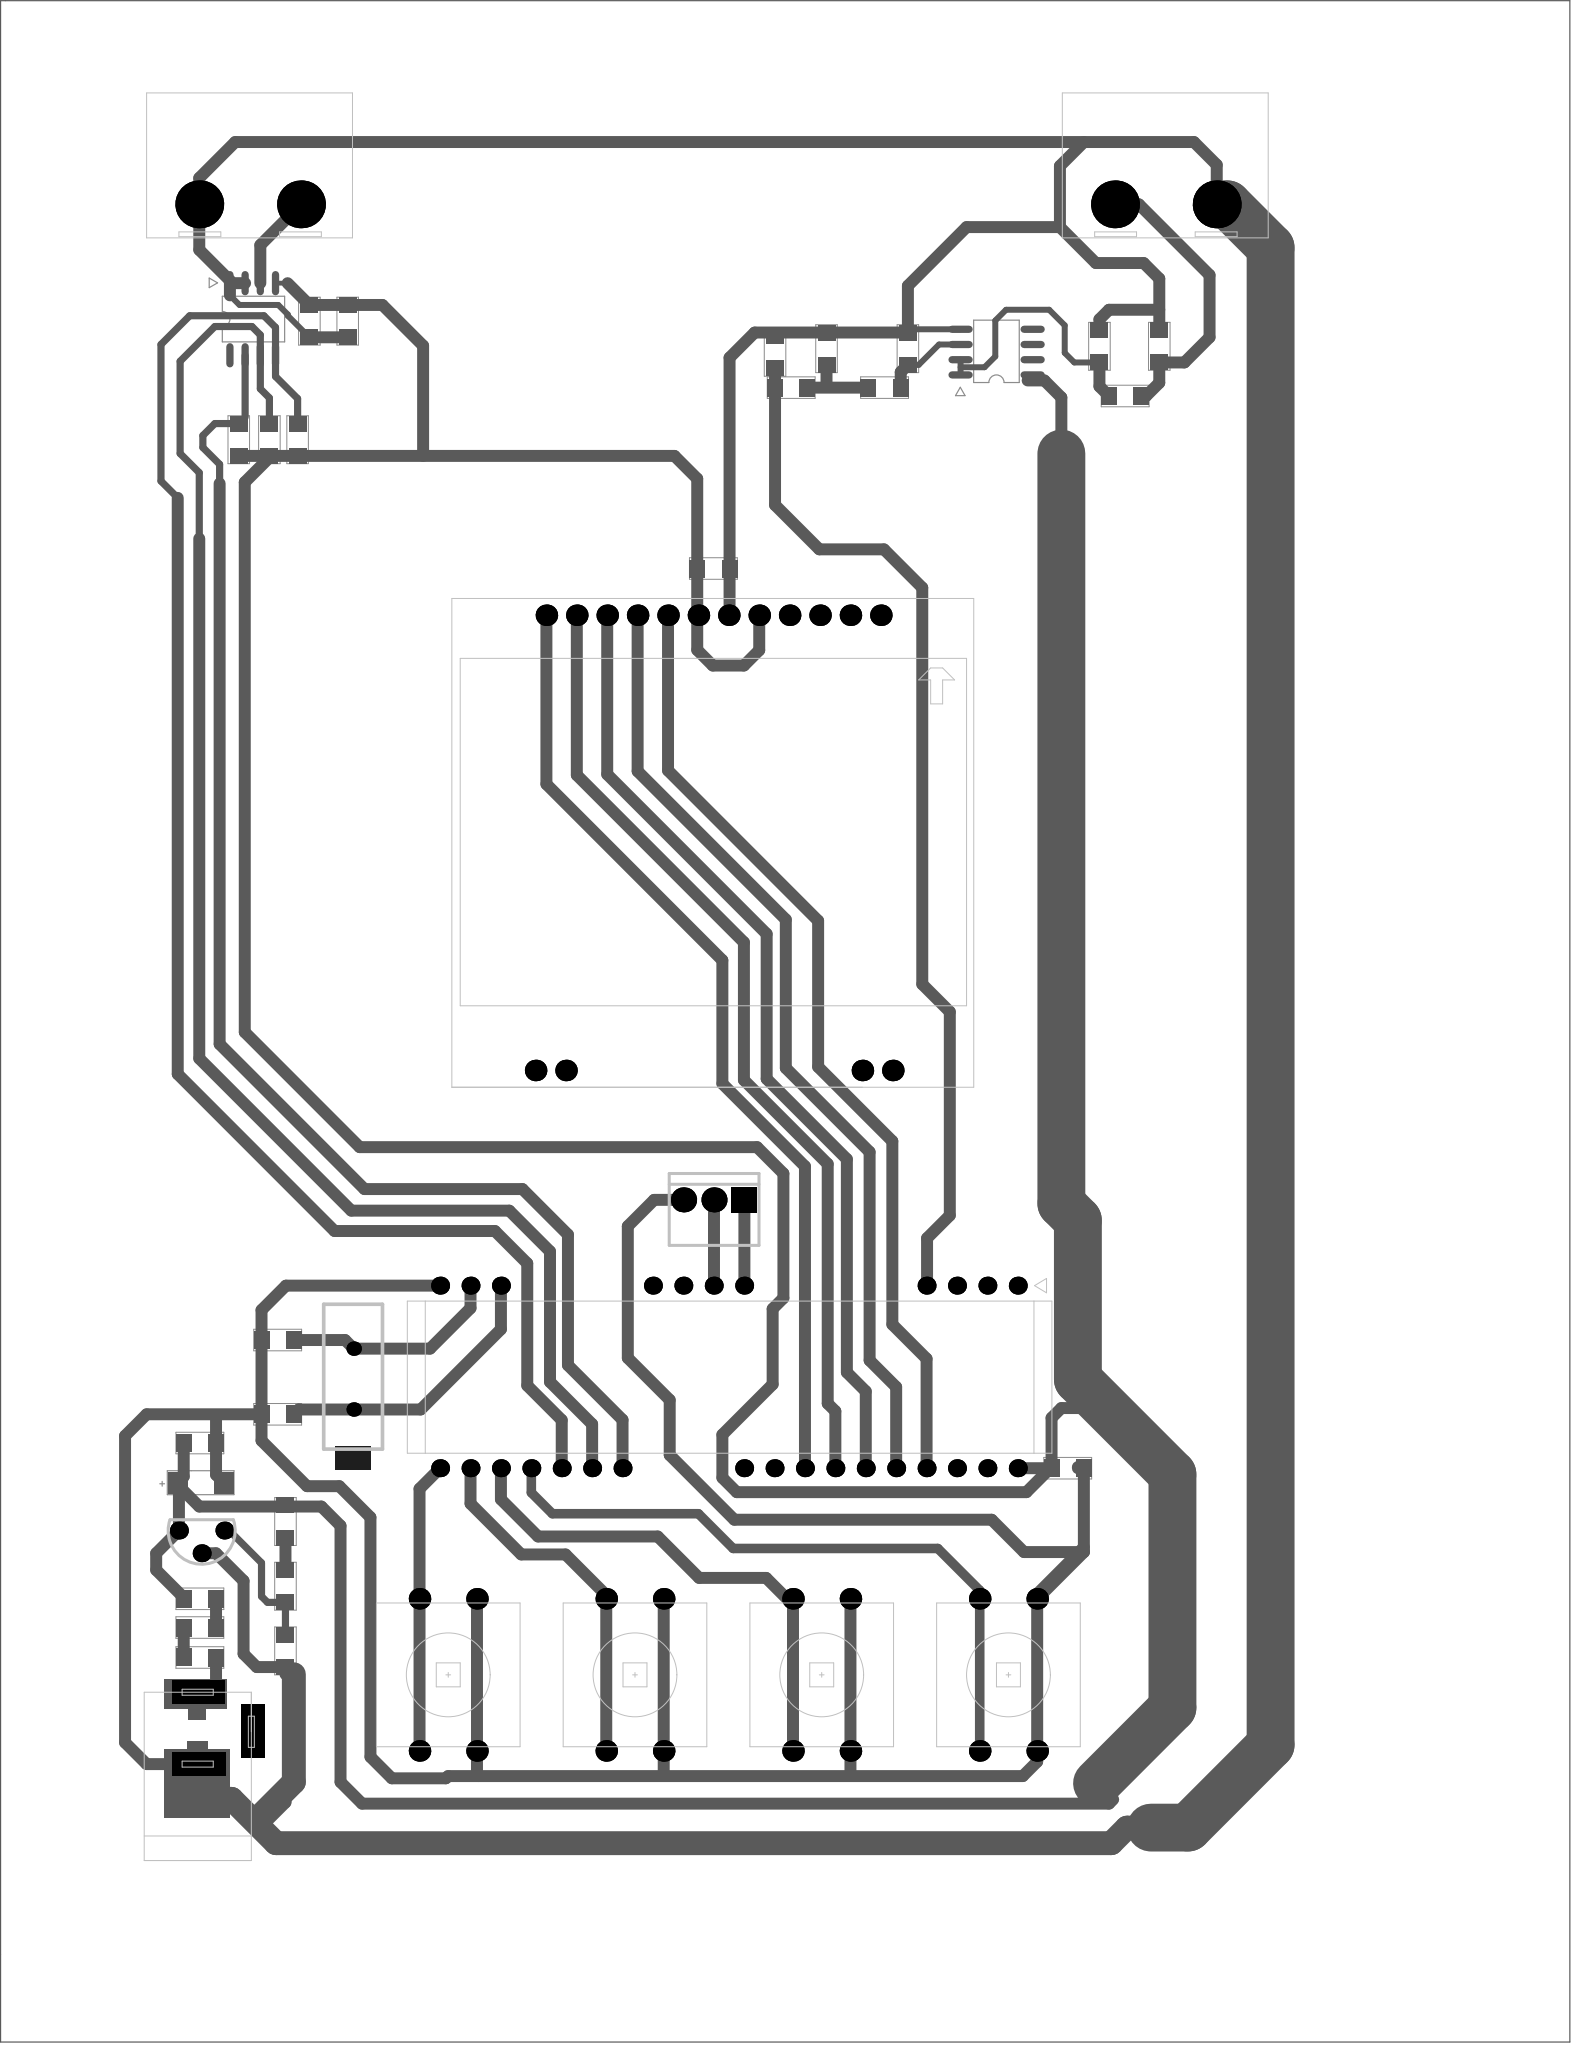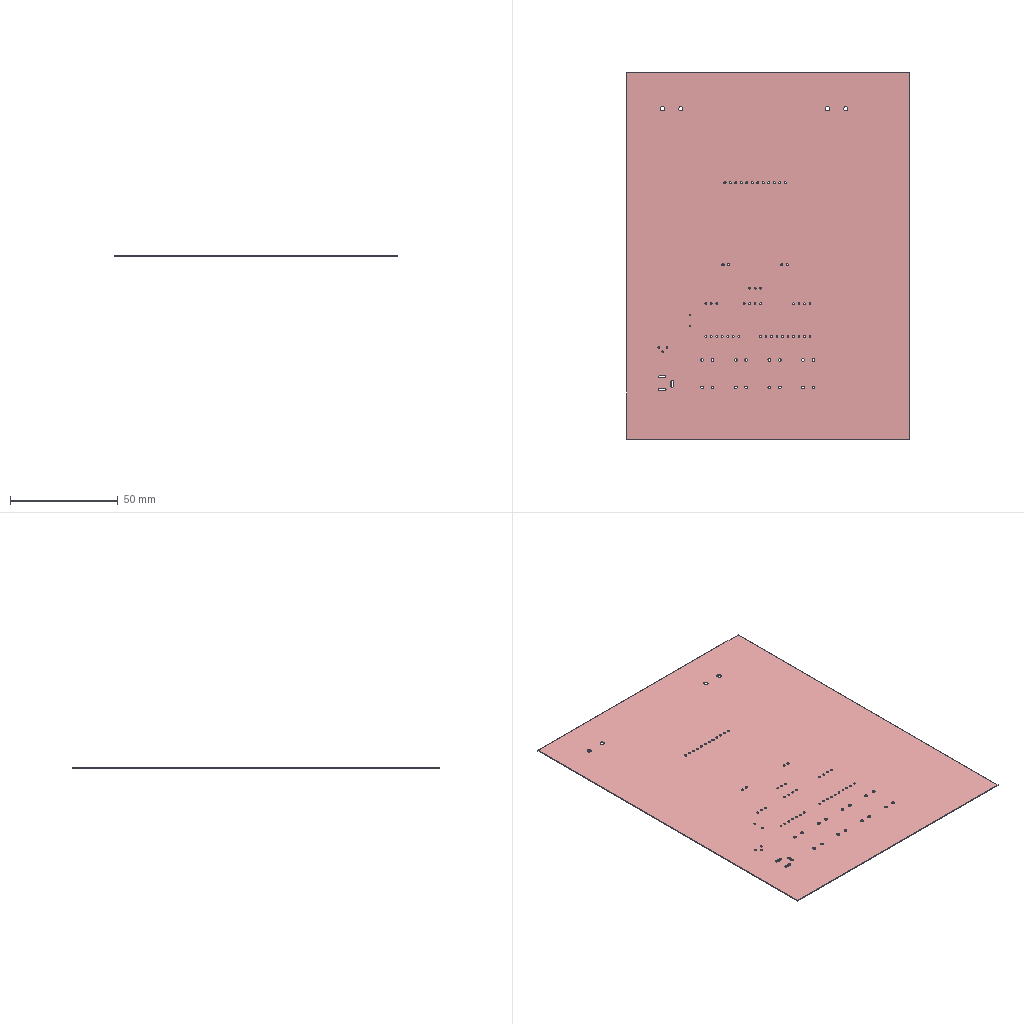Circuit board layout | Altium Designer | box 131.1 x 170.4 x 0.4 mm
Layer stack:
# Altium Designer layer stack of  (unit mm; dielectric type: 0 none, 1 core, 2 prepreg, 3 surface material)
index,name,kind,layer,copper_thickness_mm,dielectric_type,dielectric_thickness_mm,dielectric_material,dielectric_constant
0,Top Paste,other,,,,,,
1,Top Overlay,other,,,,,,
2,Top Solder,dielectric,,,3,0.0102,Solder Resist,3.5
3,Top Layer,copper,Top Layer,0.0356,,,,
4,Dielectric1,dielectric,,,0,0.32,FR-4,4.8
5,Bottom Layer,copper,Bottom Layer,0.0356,,,,
6,Bottom Solder,dielectric,,,3,0.0102,Solder Resist,3.5
7,Bottom Overlay,other,,,,,,
8,Bottom Paste,other,,,,,,
# drill layer pairs: low layer,high layer
drill_pair,Top Layer,Bottom Layer
Part placement:
Designator,Comment,Layer,Footprint,Center-X(mm),Center-Y(mm),Rotation
IC1,TL431,TopLayer,TO92,104.3,133.75,180
X1,12M,TopLayer,X,116.979,145.335,90
SW4,+,TopLayer,BUTTON/B,171.7,122.65,0
SW3,-,TopLayer,BUTTON/B,156.1,122.65,0
SW2,B,TopLayer,BUTTON/B,140.5,122.65,0
SW1,A,TopLayer,BUTTON/B,124.9,122.65,0
M1,S/12864/LCD,TopLayer,S/12864/LCD,147.12,192.1,360
J4,ISP,TopLayer,SIP3,147.1,162.3,180
J3,K/IN,TopLayer,SIP2/8.5,108.35,245.4,180
J2,0.8--4.6,TopLayer,SIP2/8.5,184.85,245.4,180
J1,J3/5V/DC/POW,TopLayer,DC/POW,105.7,118.2,270
IC3,12C5A60S2,TopLayer,DIP40,148.35,147.52,180
R14,10K,BottomLayer,0805,112.315,225.75,90
R13,10K,BottomLayer,0805,109.957,225.75,90
R5,10K,BottomLayer,0805,111.301,130.05,270
R4,10,BottomLayer,0805,111.301,135.45,270
R3,1,BottomLayer,0805,104.15,128.999,360
R2,1,BottomLayer,0805,104.15,126.601,180
R1,1,BottomLayer,0805,104.15,124.099,360
IC4,MAX6675,BottomLayer,SOP8,108.565,235.81,270
C11,22P,BottomLayer,0805,110.65,150.599,180
C10,22P,BottomLayer,0805,110.65,144.401,180
C9,104,BottomLayer,0805,113.299,235.65,270
C8,106,BottomLayer,0805,116.499,235.65,270
C7,104,BottomLayer,0805,147.05,215.001,360
C6,106,BottomLayer,0805,176.65,139.899,360
C5,106,BottomLayer,0805,184.301,233.55,90
C2,104,BottomLayer,0805,104.15,142.001,360
C1,10UF,BottomLayer,C10,104.225,138.7,360
C3,104,BottomLayer,0805,156.501,233.35,90
C4,104,BottomLayer,0805,163.299,233.35,90
IC2,LM358/rail-to-rail,BottomLayer,SOP8,170.71,233.065,360
R6,1K,BottomLayer,0805,181.45,229.401,360
R7,10K,BottomLayer,0805,153.55,230.099,360
R8,10K,BottomLayer,0805,161.35,230.101,360
R9,10K,BottomLayer,0805,111.301,124.65,270
R10,10K,BottomLayer,0805,179.301,233.55,270
R11,100K,BottomLayer,0805,152.201,233.05,270
R12,10K,BottomLayer,0805,107.399,225.75,90
Pad and via stacks:
# Altium Designer via and pad stacks of  (unit mm). Each distinct definition once, with the count of objects using it.
# via: kind,start_layer,end_layer,hole_mm,diameter_mm,mode(0 simple;1 top-mid-bottom;2 full stack),diameter_per_layer,count,example_net
# pad: kind,layer,hole_mm,hole_type(0 round;1 square;2 slot),plating,top_size,top_shape(1 round;2 rect;3 octagon;9 rounded rect),mid_size,bottom_size,mode,footprint,size_per_layer,count,example
pad,Top Layer,0,0,plated,2x3,2,2x3,2x3,0,X,,1,X1.3
pad,Bottom Layer,0,0,plated,1.5x1.3,2,1.5x1.3,1.5x1.3,0,0805,,48,R12.2
pad,Bottom Layer,0,0,plated,2.032x0.6096,1,2.032x0.6096,2.032x0.6096,0,SOP8,,16,IC4.7
pad,Bottom Layer,0,0,plated,1.6x1.8,2,1.6x1.8,1.6x1.8,0,C10,,2,C1.2
pad,Multi-Layer,0.8,0,unplated,1.5x1.5,1,1.5x1.5,1.5x1.5,0,TO92,,3,IC1.1
pad,Multi-Layer,2,0,plated,4x4,1,4x4,4x4,0,SIP2/8.5,,4,J2.2
pad,Multi-Layer,1,0,plated,2x2,2,2x2,2x2,0,DC/POW,,18,J1.3
pad,Multi-Layer,0.8,0,plated,1.5x1.5,1,1.5x1.5,1.5x1.5,0,DIP40,,28,IC3.2
pad,Multi-Layer,0.8128,0,plated,2.1x2.1,2,2.1x2.1,2.1x2.1,0,SIP3,,1,J4.1
pad,Multi-Layer,0.8128,0,plated,2.1x2.1,1,2.1x2.1,2.1x2.1,0,SIP3,,2,J4.2
pad,Multi-Layer,1.3,0,plated,1.8x1.8,1,1.8x1.8,1.8x1.8,0,BUTTON/B,,16,SW1.2
pad,Multi-Layer,1,0,plated,1.8x1.8,1,1.8x1.8,1.8x1.8,0,S/12864/LCD,,16,M1.15
pad,Multi-Layer,0.7,0,plated,1.2x1.2,1,1.2x1.2,1.2x1.2,0,X,,2,X1.2
Design rules, without the lines most boards share:
# Altium Designer design rules of  (exported by Altium Designer, unit mm)
# columns: name | kind | enabled | priority | scope1 | scope2 | descriptor | typed fields (field=value)
NetAntennae | 56 | enabled | 1 | All | All | Net Antennae (Tolerance=0mm) (All) |
SilkToSilkClearance | 55 | enabled | 1 | All | All | Silk to Silk (Clearance=0.254mm) (All),(All) |
SilkToSolderMaskClearance | 54 | enabled | 1 | IsPad | All | Silk To Solder Mask (Clearance=0.254mm) (IsPad),(All) |
MinimumSolderMaskSliver | 53 | enabled | 1 | All | All | Minimum Solder Mask Sliver (Gap=0.254mm) (All),(All) |
HoleToHoleClearance | 52 | enabled | 1 | All | All | Hole To Hole Clearance (Gap=0.254mm) (All),(All) | gap=0.254
Clearance | 0 | enabled | 1 | All | All | Clearance Constraint (Gap=0.2mm) (All),(All) | gap=0.2
PlaneConnect | 6 | enabled | 1 | All | All | Power Plane Connect Rule(Relief Connect )(Expansion=0.508mm) (Conductor Width=0.254mm) (Air Gap=0.254mm) (Entries=4) (All) | relief_conductor_width=0.254 relief_entries=4 relief_expansion=0.508
PlaneClearance | 12 | enabled | 1 | All | All | Power Plane Clearance (Clearance =0.508mm) (All) | clearance=0.508
PolygonConnect | 20 | enabled | 1 | All | All | Polygon Connect Rule(Relief Connect )(Conductor Width=0.254mm) (Relief Angle=90 Angle) (Entries=4) (Air Gap Width=0.254mm) (All),(All) | connect_style(0=relief,1=direct,2=none)=0 relief_conductor_width=0.254 relief_entries=4
Width | 2 | enabled | 1 | All | All | Width Constraint (Min=0.254mm) (Max=9mm) (Preferred=0.3mm) (All) |
RoutingCorners | 10 | enabled | 1 | All | All | Routing Corners (Style=45-Degree) (Min Setback=2.54mm) (Max Setback=2.54mm) (All) |
RoutingVias | 11 | enabled | 1 | All | All | Routing Via (MinHoleWidth=0.711mm) (MaxHoleWidth=9mm) (PreferredHoleWidth=0.711mm) (MinWidth=1.27mm) (MaxWidth=9mm) (PreferedWidth=1.27mm) (All) | via_min_hole=0.711 via_max_hole=9 via_preferred_diameter=1.27 via_preferred_hole=0.711
PasteMaskExpansion | 14 | enabled | 1 | All | All | Paste Mask Expansion (Expansion =0mm) (All) | expansion=0
SolderMaskExpansion | 13 | enabled | 1 | All | All | Solder Mask Expansion (Expansion =0.102mm) (All) | expansion=0.1016
TestPointUsage | 44 | enabled | 1 | All | All | Fabrication Testpoint Usage (Valid =One Required, Allow multiple per net=No) (All) |
Testpoint | 43 | enabled | 1 | All | All | Fabrication Testpoint Style (Under Component=Yes) (All) |
ComponentClearance | 24 | enabled | 1 | All | All | Component Clearance Constraint ( Horizontal Gap = 0.254mm, Vertical Gap = 0.254mm ) (All),(All)  | gap=0.254
Height | 50 | enabled | 1 | All | All | Height Constraint (Min=0mm) (Max=25.4mm) (Prefered=12.7mm) (All) | min_height=0 max_height=25.4
HoleSize | 42 | enabled | 1 | All | All | Hole Size Constraint (Min=0.025mm) (Max=2.54mm) (All) |
DiffPairsRouting | 51 | enabled | 1 | All | All | Differential Pairs Uncoupled Length using the Gap Constraints (Min=0.254mm) (Max=0.254mm) (Prefered=0.254mm)  and Width Constraints (Min=0.381mm) (Max=0.381mm) (Prefered=0.381mm) (All) |
Classes set for this board:
# Altium Designer classes of  (member kind: 0 net, 1 component, 2 from-to, 3 pad, 4 layer, 5 differential pair, 6 design channel, 7 polygon, 8 structure, 9 xSignal)
# columns: class name | member kind | superclass | members
Sheet1 | 1 | no | C1; C2; C5; C6; C7; C8; C9; C10; C11; IC1; IC3; IC4; J1; J2; J3; J4; M1; R1; R2; R3; R4; R5; R13; R14; SW1; SW2; SW3; SW4; X1; SW1; SW2; SW3; SW4; C1; C2; C5; C6; C7; C8; C9; C10; C11; IC1; IC3; IC4; J1; J2; J3; J4; M1; R1; R2; R3; R4; R5; R13; R14; SW1; SW2; SW3; SW4; X1; C10; C11; IC4; R8; R9; R10; R11; R12; R13; R14;